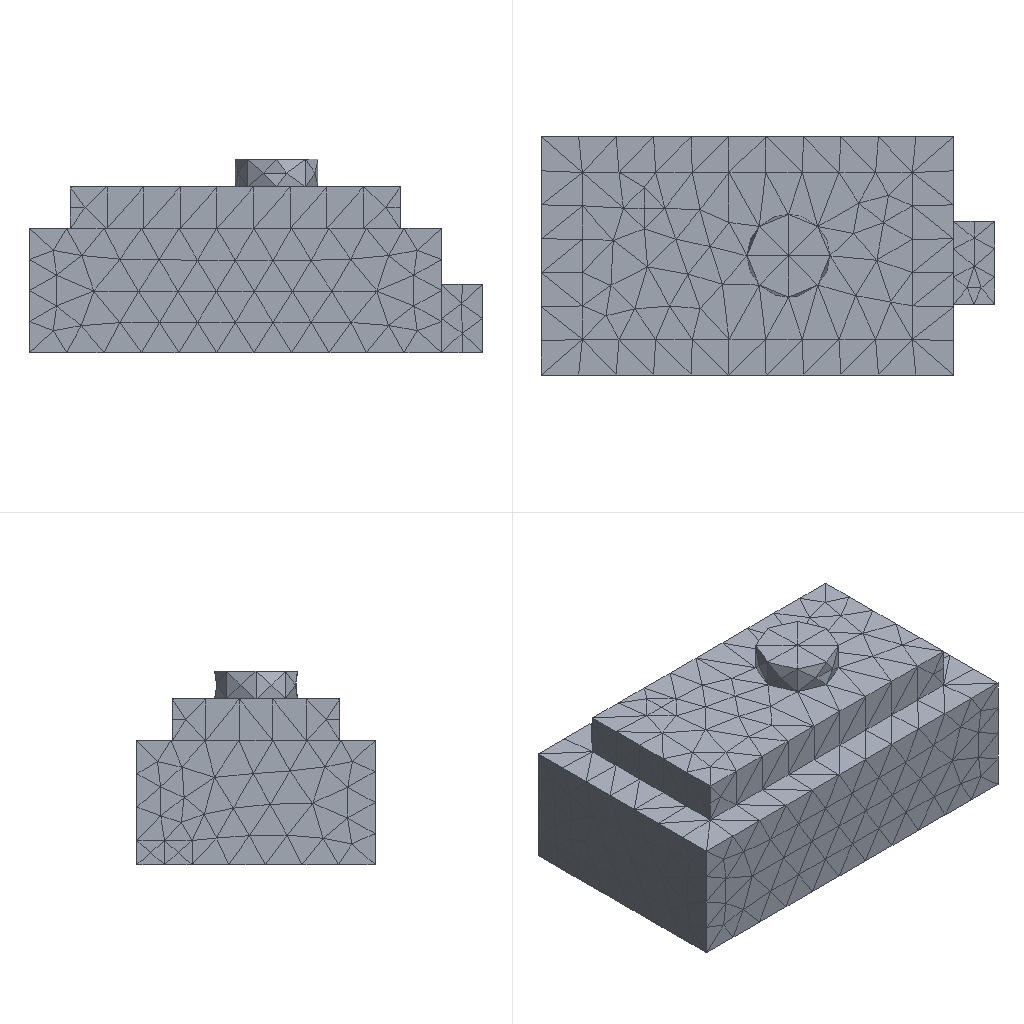Simulation study | ansys mapdl
Set-up summary:
category,name,step,type,value,unit,region
solver,ansys_mapdl
units,mm-N-s-tonne (MPa),,inferred,E=210000 density=
analysis,model,,static
mesh,nodes,,,4454
mesh,elements,,,2638
element_type,SOLID187,,,2638
material,mat 1,,E,210000
material,mat 1,,nu,0.3
load,,model,body load temp,,,all
load,,model,force,"1000 [dir=(0, 0, -1) n=315]",,node list
bc,,model,fixed,"[dofs=UX,UY,UZ n=5060]",,node list
Ansys APDL input file, long lists of numbers shortened:
/COM,ANSYS RELEASE 2026 R1           BUILD 26.1      UP20260202       09:10:33
/PREP7
/NOPR
/TITLE,2
ANTYPE, 0
*IF,_CDRDOFF,EQ,1,THEN     !if solid model was read in
_CDRDOFF=             !reset flag, numoffs already performed
*ELSE              !offset database for the following FE model
NUMOFF,NODE,     4454
NUMOFF,ELEM,     2638
NUMOFF,MAT ,        1
NUMOFF,TYPE,        1
*ENDIF
*SET,_RETURN ,  0.
*SET,_STATUS ,  0.
*SET,_UIQR   ,  315.
*SET,__FLOATPARAMETER__,  4454.
DOF,DELETE
ETBLOCK,        1,        1
(2i9,19a9)
        1      187        0        0        0        0        0        0        0        0        0        0        0        0        0        0        0        0        0        0        0
       -1
NBLOCK,6,SOLID,      4454,      4454
(3i9,6e21.13e3)
        1        0        0-4.3700000000000E+001 3.4500000000000E+001 7.0000000000000E+000
! (4453 more lines like these left out)
N,UNBL,LOC,       -1,
EBLOCK,19,SOLID,      2638,      2638
(19i10)
         1         1         1         1         0         0         0         0        10         0         1      1775      1776      1777      1778      2017      2018      2019      2020
! (5275 more lines like these left out)
        -1
MPTEMP,UNBL, 1, 1,  0.    ,
MPDATA,UNBL, 1,EX  ,       1, 1,  210000.000    ,
MPTEMP,UNBL, 1, 1,  0.    ,
MPDATA,UNBL, 1,NUXY,       1, 1, 0.3    ,
MPTEMP,UNBL, 1, 1,  0.    ,
MPDATA,UNBL, 1,PRXY,       1, 1, 0.3    ,
EXTOPT,ATTR,      0,      0,      0
EXTOPT,ESIZE,  0,  0.
EXTOPT,ACLEAR,      0
TREF,  0.
IRLF,  0
BFUNIF,TEMP,_TINY
ACEL,  0.    ,  0.    ,  0.
OMEGA,  0.    ,  0.    ,  0.
DOMEGA,  0.    ,  0.    ,  0.
CGLOC,  0.    ,  0.    ,  0.
CGOMEGA,  0.    ,  0.    ,  0.
DCGOMG,  0.    ,  0.    ,  0.
KUSE,     0
TIME,  0.
ALPHAD,  0.
BETAD,  0.
DMPRAT,  0.
DMPSTR,  0.
CRPLIM, 0.1    ,   0
CRPLIM,  0.    ,   1
NCNV,     0, 1.000000000E+12,     0,  0.    ,  0.
NEQIT,     0
ERESX,DEFA
DBLOCK,      5060
(i9,a6,2(pg16.9))
        1  UX    0.00000000      0.00000000
! (5059 more lines like these left out)
       -1
FBLOCK,       315
(i9,a6,2(pg16.9))
      589  FZ   -3.17460317      0.00000000
! (314 more lines like these left out)
       -1
/GO
FINISH
Results summary:
result,analysis_type_db,,,static,unstated
result,n_sets,,,1,unstated
result,load_steps[0].set,load_step=1,,1,unstated
result,load_steps[0].substep,load_step=1,,1,unstated
result,load_steps[0].time,load_step=1,,1,unstated
result,load_steps[0].freq,load_step=1,,1,unstated
result,load_steps[0].max_usum,load_step=1,,9.43814e-05,unstated
result,load_steps[0].max_seqv,load_step=1,,1.026,unstated
result,load_steps[0].reaction_sum.FX,load_step=1,,1.88294e-13,unstated
result,load_steps[0].reaction_sum.FY,load_step=1,,9.79483e-12,unstated
result,load_steps[0].reaction_sum.FZ,load_step=1,,1000,unstated
result,load_steps[0].reaction_sum.MX,load_step=1,,0,unstated
result,load_steps[0].reaction_sum.MY,load_step=1,,0,unstated
result,load_steps[0].reaction_sum.MZ,load_step=1,,0,unstated
result,convergence,,,results present for all listed sets,unstated